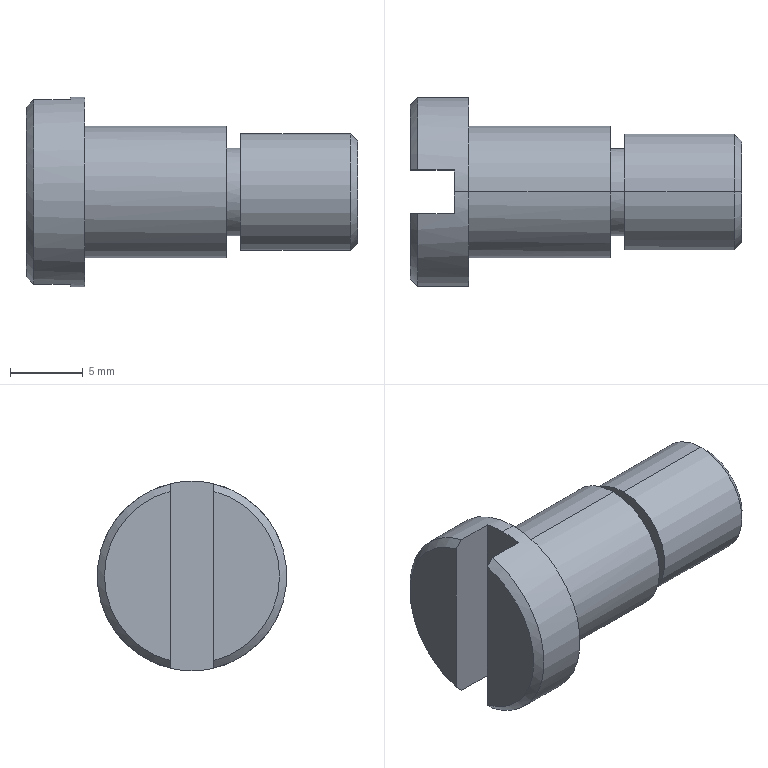Part | STEP file | 101000007761 | 1 solid | 21 faces | box 22.7 x 13 x 13 mm | volume 1455 mm3 | plane 9 | cylinder 8 | cone 4 | commonest cylinder face diameters 6 x2 8 x2 9 x2 13 x2
STEP:
#1=CARTESIAN_POINT('',(-23.823,0.,-3.5));
#2=VERTEX_POINT('',#1);
#3=CARTESIAN_POINT('',(-23.823,0.,3.5));
#4=VERTEX_POINT('',#3);
#5=CARTESIAN_POINT('',(-23.823,0.,0.));
#6=DIRECTION('',(-1.,0.,0.));
#7=AXIS2_PLACEMENT_3D('',#5,#6,$);
#8=CIRCLE('',#7,3.5);
#9=EDGE_CURVE('',#2,#4,#8,.F.);
#10=ORIENTED_EDGE('',*,*,#9,.F.);
#11=CARTESIAN_POINT('',(-24.323,0.,-4.));
#12=VERTEX_POINT('',#11);
#13=CARTESIAN_POINT('',(-353575.714,0.,-353555.391));
#14=DIRECTION('',(-0.7071,0.,-0.7071));
#15=VECTOR('',#14,1.);
#16=LINE('',#13,#15);
#17=EDGE_CURVE('',#2,#12,#16,.T.);
#18=ORIENTED_EDGE('',*,*,#17,.T.);
#19=CARTESIAN_POINT('',(-24.323,0.,4.));
#20=VERTEX_POINT('',#19);
#21=CARTESIAN_POINT('',(-24.323,0.,0.));
#22=DIRECTION('',(-1.,0.,0.));
#23=AXIS2_PLACEMENT_3D('',#21,#22,$);
#24=CIRCLE('',#23,4.);
#25=EDGE_CURVE('',#20,#12,#24,.T.);
#26=ORIENTED_EDGE('',*,*,#25,.F.);
#27=CARTESIAN_POINT('',(-353575.714,0.,353555.391));
#28=DIRECTION('',(-0.7071,0.,0.7071));
#29=VECTOR('',#28,1.);
#30=LINE('',#27,#29);
#31=EDGE_CURVE('',#4,#20,#30,.T.);
#32=ORIENTED_EDGE('',*,*,#31,.F.);
#33=EDGE_LOOP('',(#10,#18,#26,#32));
#34=FACE_OUTER_BOUND('',#33,.T.);
#35=CARTESIAN_POINT('',(-24.323,0.,0.));
#36=DIRECTION('',(-1.,0.,0.));
#37=DIRECTION('',(0.,0.,1.));
#38=AXIS2_PLACEMENT_3D('',#35,#36,#37);
#39=CONICAL_SURFACE('',#38,4.,0.7854);
#40=ADVANCED_FACE('',(#34),#39,.T.);
#41=CARTESIAN_POINT('',(-23.823,0.,3.5));
#42=CARTESIAN_POINT('',(-23.823,-0.3666,3.5));
#43=CARTESIAN_POINT('',(-23.823,-0.7332,3.452));
#44=CARTESIAN_POINT('',(-23.823,-1.091,3.356));
#45=CARTESIAN_POINT('',(-23.823,-1.774,3.072));
#46=CARTESIAN_POINT('',(-23.823,-2.361,2.623));
#47=CARTESIAN_POINT('',(-23.823,-2.624,2.36));
#48=CARTESIAN_POINT('',(-23.823,-3.073,1.773));
#49=CARTESIAN_POINT('',(-23.823,-3.356,1.09));
#50=CARTESIAN_POINT('',(-23.823,-3.452,0.7319));
#51=CARTESIAN_POINT('',(-23.823,-3.548,-0.001322));
#52=CARTESIAN_POINT('',(-23.823,-3.452,-0.7345));
#53=CARTESIAN_POINT('',(-23.823,-3.356,-1.093));
#54=CARTESIAN_POINT('',(-23.823,-3.072,-1.776));
#55=CARTESIAN_POINT('',(-23.823,-2.622,-2.362));
#56=CARTESIAN_POINT('',(-23.823,-2.359,-2.624));
#57=CARTESIAN_POINT('',(-23.823,-1.773,-3.073));
#58=CARTESIAN_POINT('',(-23.823,-1.09,-3.356));
#59=CARTESIAN_POINT('',(-23.823,-0.7322,-3.452));
#60=CARTESIAN_POINT('',(-23.823,-0.3661,-3.5));
#61=CARTESIAN_POINT('',(-23.823,0.,-3.5));
#62=B_SPLINE_CURVE_WITH_KNOTS('',5,(#41,#42,#43,#44,#45,#46,#47,#48,#49,#50,#51,#52,#53,#54,#55,#56,#57,#58,#59,#60,#61),.UNSPECIFIED.,.F.,.U.,(6,3,3,3,3,3,6),(0.,2.592,5.185,7.777,10.369,12.961,15.55),.UNSPECIFIED.);
#63=EDGE_CURVE('',#4,#2,#62,.T.);
#64=ORIENTED_EDGE('',*,*,#63,.T.);
#65=ORIENTED_EDGE('',*,*,#9,.T.);
#66=EDGE_LOOP('',(#64,#65));
#67=FACE_OUTER_BOUND('',#66,.T.);
#68=CARTESIAN_POINT('',(-23.823,4.,0.));
#69=DIRECTION('',(-1.,0.,0.));
#70=DIRECTION('',(0.,0.,1.));
#71=AXIS2_PLACEMENT_3D('',#68,#69,#70);
#72=PLANE('',#71);
#73=ADVANCED_FACE('',(#67),#72,.F.);
#74=ORIENTED_EDGE('',*,*,#17,.F.);
#75=ORIENTED_EDGE('',*,*,#63,.F.);
#76=ORIENTED_EDGE('',*,*,#31,.T.);
#77=CARTESIAN_POINT('',(-24.323,0.,0.));
#78=DIRECTION('',(-1.,0.,0.));
#79=AXIS2_PLACEMENT_3D('',#77,#78,$);
#80=CIRCLE('',#79,4.);
#81=EDGE_CURVE('',#12,#20,#80,.T.);
#82=ORIENTED_EDGE('',*,*,#81,.F.);
#83=EDGE_LOOP('',(#74,#75,#76,#82));
#84=FACE_OUTER_BOUND('',#83,.T.);
#85=CARTESIAN_POINT('',(-24.323,0.,0.));
#86=DIRECTION('',(-1.,0.,0.));
#87=DIRECTION('',(0.,0.,-1.));
#88=AXIS2_PLACEMENT_3D('',#85,#86,#87);
#89=CONICAL_SURFACE('',#88,4.,0.7854);
#90=ADVANCED_FACE('',(#84),#89,.T.);
#91=ORIENTED_EDGE('',*,*,#25,.T.);
#92=CARTESIAN_POINT('',(-31.823,0.,-4.));
#93=VERTEX_POINT('',#92);
#94=CARTESIAN_POINT('',(-55.053,0.,-4.));
#95=DIRECTION('',(-1.,0.,0.));
#96=VECTOR('',#95,1.);
#97=LINE('',#94,#96);
#98=EDGE_CURVE('',#12,#93,#97,.T.);
#99=ORIENTED_EDGE('',*,*,#98,.T.);
#100=CARTESIAN_POINT('',(-31.823,0.,4.));
#101=VERTEX_POINT('',#100);
#102=CARTESIAN_POINT('',(-31.823,0.,0.));
#103=DIRECTION('',(-1.,0.,0.));
#104=AXIS2_PLACEMENT_3D('',#102,#103,$);
#105=CIRCLE('',#104,4.);
#106=EDGE_CURVE('',#101,#93,#105,.T.);
#107=ORIENTED_EDGE('',*,*,#106,.F.);
#108=CARTESIAN_POINT('',(-55.053,0.,4.));
#109=DIRECTION('',(-1.,0.,0.));
#110=VECTOR('',#109,1.);
#111=LINE('',#108,#110);
#112=EDGE_CURVE('',#20,#101,#111,.T.);
#113=ORIENTED_EDGE('',*,*,#112,.F.);
#114=EDGE_LOOP('',(#91,#99,#107,#113));
#115=FACE_OUTER_BOUND('',#114,.T.);
#116=CARTESIAN_POINT('',(-55.053,0.,0.));
#117=DIRECTION('',(-1.,0.,0.));
#118=DIRECTION('',(0.,0.,1.));
#119=AXIS2_PLACEMENT_3D('',#116,#117,#118);
#120=CYLINDRICAL_SURFACE('',#119,4.);
#121=ADVANCED_FACE('',(#115),#120,.T.);
#122=ORIENTED_EDGE('',*,*,#98,.F.);
#123=ORIENTED_EDGE('',*,*,#81,.T.);
#124=ORIENTED_EDGE('',*,*,#112,.T.);
#125=CARTESIAN_POINT('',(-31.823,0.,-4.));
#126=CARTESIAN_POINT('',(-31.823,-0.6283,-4.));
#127=CARTESIAN_POINT('',(-31.823,-1.257,-3.877));
#128=CARTESIAN_POINT('',(-31.823,-1.853,-3.63));
#129=CARTESIAN_POINT('',(-31.823,-2.916,-2.916));
#130=CARTESIAN_POINT('',(-31.823,-3.63,-1.853));
#131=CARTESIAN_POINT('',(-31.823,-3.877,-1.257));
#132=CARTESIAN_POINT('',(-31.823,-4.123,0.));
#133=CARTESIAN_POINT('',(-31.823,-3.877,1.257));
#134=CARTESIAN_POINT('',(-31.823,-3.63,1.853));
#135=CARTESIAN_POINT('',(-31.823,-2.916,2.916));
#136=CARTESIAN_POINT('',(-31.823,-1.853,3.63));
#137=CARTESIAN_POINT('',(-31.823,-1.257,3.877));
#138=CARTESIAN_POINT('',(-31.823,-0.6283,4.));
#139=CARTESIAN_POINT('',(-31.823,0.,4.));
#140=B_SPLINE_CURVE_WITH_KNOTS('',5,(#125,#126,#127,#128,#129,#130,#131,#132,#133,#134,#135,#136,#137,#138,#139),.UNSPECIFIED.,.F.,.U.,(6,3,3,3,6),(-6.283,-3.142,0.,3.142,6.283),.UNSPECIFIED.);
#141=EDGE_CURVE('',#93,#101,#140,.T.);
#142=ORIENTED_EDGE('',*,*,#141,.F.);
#143=EDGE_LOOP('',(#122,#123,#124,#142));
#144=FACE_OUTER_BOUND('',#143,.T.);
#145=CARTESIAN_POINT('',(-55.053,0.,0.));
#146=DIRECTION('',(-1.,0.,0.));
#147=DIRECTION('',(0.,0.,-1.));
#148=AXIS2_PLACEMENT_3D('',#145,#146,#147);
#149=CYLINDRICAL_SURFACE('',#148,4.);
#150=ADVANCED_FACE('',(#144),#149,.T.);
#151=ORIENTED_EDGE('',*,*,#106,.T.);
#152=ORIENTED_EDGE('',*,*,#141,.T.);
#153=EDGE_LOOP('',(#151,#152));
#154=FACE_OUTER_BOUND('',#153,.T.);
#155=CARTESIAN_POINT('',(-31.823,0.,3.));
#156=VERTEX_POINT('',#155);
#157=CARTESIAN_POINT('',(-31.823,0.,-3.));
#158=VERTEX_POINT('',#157);
#159=CARTESIAN_POINT('',(-31.823,0.,3.));
#160=CARTESIAN_POINT('',(-31.823,0.3394,3.));
#161=CARTESIAN_POINT('',(-31.823,0.6788,2.952));
#162=CARTESIAN_POINT('',(-31.823,1.009,2.856));
#163=CARTESIAN_POINT('',(-31.823,1.634,2.573));
#164=CARTESIAN_POINT('',(-31.823,2.155,2.128));
#165=CARTESIAN_POINT('',(-31.823,2.383,1.87));
#166=CARTESIAN_POINT('',(-31.823,2.758,1.297));
#167=CARTESIAN_POINT('',(-31.823,2.96,0.6415));
#168=CARTESIAN_POINT('',(-31.823,3.014,0.3017));
#169=CARTESIAN_POINT('',(-31.823,3.024,-0.3838));
#170=CARTESIAN_POINT('',(-31.823,2.843,-1.045));
#171=CARTESIAN_POINT('',(-31.823,2.706,-1.361));
#172=CARTESIAN_POINT('',(-31.823,2.347,-1.945));
#173=CARTESIAN_POINT('',(-31.823,1.84,-2.406));
#174=CARTESIAN_POINT('',(-31.823,1.555,-2.599));
#175=CARTESIAN_POINT('',(-31.823,1.077,-2.833));
#176=CARTESIAN_POINT('',(-31.823,0.5622,-2.956));
#177=CARTESIAN_POINT('',(-31.823,0.3758,-2.985));
#178=CARTESIAN_POINT('',(-31.823,0.1879,-3.));
#179=CARTESIAN_POINT('',(-31.823,0.,-3.));
#180=B_SPLINE_CURVE_WITH_KNOTS('',5,(#159,#160,#161,#162,#163,#164,#165,#166,#167,#168,#169,#170,#171,#172,#173,#174,#175,#176,#177,#178,#179),.UNSPECIFIED.,.F.,.U.,(6,3,3,3,3,3,6),(0.,2.4,4.8,7.2,9.6,12.,13.328),.UNSPECIFIED.);
#181=EDGE_CURVE('',#156,#158,#180,.T.);
#182=ORIENTED_EDGE('',*,*,#181,.F.);
#183=CARTESIAN_POINT('',(-31.823,0.,-3.));
#184=CARTESIAN_POINT('',(-31.823,-0.3394,-3.));
#185=CARTESIAN_POINT('',(-31.823,-0.6788,-2.952));
#186=CARTESIAN_POINT('',(-31.823,-1.009,-2.856));
#187=CARTESIAN_POINT('',(-31.823,-1.634,-2.573));
#188=CARTESIAN_POINT('',(-31.823,-2.155,-2.128));
#189=CARTESIAN_POINT('',(-31.823,-2.383,-1.87));
#190=CARTESIAN_POINT('',(-31.823,-2.758,-1.297));
#191=CARTESIAN_POINT('',(-31.823,-2.96,-0.6415));
#192=CARTESIAN_POINT('',(-31.823,-3.014,-0.3017));
#193=CARTESIAN_POINT('',(-31.823,-3.024,0.3838));
#194=CARTESIAN_POINT('',(-31.823,-2.843,1.045));
#195=CARTESIAN_POINT('',(-31.823,-2.706,1.361));
#196=CARTESIAN_POINT('',(-31.823,-2.347,1.945));
#197=CARTESIAN_POINT('',(-31.823,-1.84,2.406));
#198=CARTESIAN_POINT('',(-31.823,-1.555,2.599));
#199=CARTESIAN_POINT('',(-31.823,-1.077,2.833));
#200=CARTESIAN_POINT('',(-31.823,-0.5622,2.956));
#201=CARTESIAN_POINT('',(-31.823,-0.3758,2.985));
#202=CARTESIAN_POINT('',(-31.823,-0.1879,3.));
#203=CARTESIAN_POINT('',(-31.823,0.,3.));
#204=B_SPLINE_CURVE_WITH_KNOTS('',5,(#183,#184,#185,#186,#187,#188,#189,#190,#191,#192,#193,#194,#195,#196,#197,#198,#199,#200,#201,#202,#203),.UNSPECIFIED.,.F.,.U.,(6,3,3,3,3,3,6),(0.,2.4,4.8,7.2,9.6,12.,13.328),.UNSPECIFIED.);
#205=EDGE_CURVE('',#158,#156,#204,.T.);
#206=ORIENTED_EDGE('',*,*,#205,.F.);
#207=EDGE_LOOP('',(#182,#206));
#208=FACE_BOUND('',#207,.T.);
#209=CARTESIAN_POINT('',(-31.823,3.,0.));
#210=DIRECTION('',(1.,0.,0.));
#211=DIRECTION('',(0.,0.,-1.));
#212=AXIS2_PLACEMENT_3D('',#209,#210,#211);
#213=PLANE('',#212);
#214=ADVANCED_FACE('',(#154,#208),#213,.F.);
#215=ORIENTED_EDGE('',*,*,#181,.T.);
#216=CARTESIAN_POINT('',(-32.823,0.,-3.));
#217=VERTEX_POINT('',#216);
#218=CARTESIAN_POINT('',(-55.053,0.,-3.));
#219=DIRECTION('',(-1.,0.,0.));
#220=VECTOR('',#219,1.);
#221=LINE('',#218,#220);
#222=EDGE_CURVE('',#158,#217,#221,.T.);
#223=ORIENTED_EDGE('',*,*,#222,.T.);
#224=CARTESIAN_POINT('',(-32.823,0.,3.));
#225=VERTEX_POINT('',#224);
#226=CARTESIAN_POINT('',(-32.823,0.,0.));
#227=DIRECTION('',(-1.,0.,0.));
#228=AXIS2_PLACEMENT_3D('',#226,#227,$);
#229=CIRCLE('',#228,3.);
#230=EDGE_CURVE('',#225,#217,#229,.T.);
#231=ORIENTED_EDGE('',*,*,#230,.F.);
#232=CARTESIAN_POINT('',(-55.053,0.,3.));
#233=DIRECTION('',(-1.,0.,0.));
#234=VECTOR('',#233,1.);
#235=LINE('',#232,#234);
#236=EDGE_CURVE('',#156,#225,#235,.T.);
#237=ORIENTED_EDGE('',*,*,#236,.F.);
#238=EDGE_LOOP('',(#215,#223,#231,#237));
#239=FACE_OUTER_BOUND('',#238,.T.);
#240=CARTESIAN_POINT('',(-55.053,0.,0.));
#241=DIRECTION('',(-1.,0.,0.));
#242=DIRECTION('',(0.,0.,1.));
#243=AXIS2_PLACEMENT_3D('',#240,#241,#242);
#244=CYLINDRICAL_SURFACE('',#243,3.);
#245=ADVANCED_FACE('',(#239),#244,.T.);
#246=ORIENTED_EDGE('',*,*,#222,.F.);
#247=ORIENTED_EDGE('',*,*,#205,.T.);
#248=ORIENTED_EDGE('',*,*,#236,.T.);
#249=CARTESIAN_POINT('',(-32.823,0.,-3.));
#250=CARTESIAN_POINT('',(-32.823,-0.9425,-3.));
#251=CARTESIAN_POINT('',(-32.823,-1.885,-2.63));
#252=CARTESIAN_POINT('',(-32.823,-2.63,-1.885));
#253=CARTESIAN_POINT('',(-32.823,-3.37,0.));
#254=CARTESIAN_POINT('',(-32.823,-2.63,1.885));
#255=CARTESIAN_POINT('',(-32.823,-1.885,2.63));
#256=CARTESIAN_POINT('',(-32.823,-0.9425,3.));
#257=CARTESIAN_POINT('',(-32.823,0.,3.));
#258=B_SPLINE_CURVE_WITH_KNOTS('',5,(#249,#250,#251,#252,#253,#254,#255,#256,#257),.UNSPECIFIED.,.F.,.U.,(6,3,6),(-4.712,0.,4.712),.UNSPECIFIED.);
#259=EDGE_CURVE('',#217,#225,#258,.T.);
#260=ORIENTED_EDGE('',*,*,#259,.F.);
#261=EDGE_LOOP('',(#246,#247,#248,#260));
#262=FACE_OUTER_BOUND('',#261,.T.);
#263=CARTESIAN_POINT('',(-55.053,0.,0.));
#264=DIRECTION('',(-1.,0.,0.));
#265=DIRECTION('',(0.,0.,-1.));
#266=AXIS2_PLACEMENT_3D('',#263,#264,#265);
#267=CYLINDRICAL_SURFACE('',#266,3.);
#268=ADVANCED_FACE('',(#262),#267,.T.);
#269=CARTESIAN_POINT('',(-32.823,0.,4.5));
#270=VERTEX_POINT('',#269);
#271=CARTESIAN_POINT('',(-32.823,0.,-4.5));
#272=VERTEX_POINT('',#271);
#273=CARTESIAN_POINT('',(-32.823,0.,0.));
#274=DIRECTION('',(-1.,0.,0.));
#275=AXIS2_PLACEMENT_3D('',#273,#274,$);
#276=CIRCLE('',#275,4.5);
#277=EDGE_CURVE('',#270,#272,#276,.T.);
#278=ORIENTED_EDGE('',*,*,#277,.F.);
#279=CARTESIAN_POINT('',(-32.823,0.,0.));
#280=DIRECTION('',(-1.,0.,0.));
#281=AXIS2_PLACEMENT_3D('',#279,#280,$);
#282=CIRCLE('',#281,4.5);
#283=EDGE_CURVE('',#272,#270,#282,.T.);
#284=ORIENTED_EDGE('',*,*,#283,.F.);
#285=EDGE_LOOP('',(#278,#284));
#286=FACE_OUTER_BOUND('',#285,.T.);
#287=ORIENTED_EDGE('',*,*,#230,.T.);
#288=ORIENTED_EDGE('',*,*,#259,.T.);
#289=EDGE_LOOP('',(#287,#288));
#290=FACE_BOUND('',#289,.T.);
#291=CARTESIAN_POINT('',(-32.823,4.5,0.));
#292=DIRECTION('',(-1.,0.,0.));
#293=DIRECTION('',(0.,0.,1.));
#294=AXIS2_PLACEMENT_3D('',#291,#292,#293);
#295=PLANE('',#294);
#296=ADVANCED_FACE('',(#286,#290),#295,.F.);
#297=ORIENTED_EDGE('',*,*,#277,.T.);
#298=CARTESIAN_POINT('',(-42.523,0.,-4.5));
#299=VERTEX_POINT('',#298);
#300=CARTESIAN_POINT('',(-55.053,0.,-4.5));
#301=DIRECTION('',(-1.,0.,0.));
#302=VECTOR('',#301,1.);
#303=LINE('',#300,#302);
#304=EDGE_CURVE('',#272,#299,#303,.T.);
#305=ORIENTED_EDGE('',*,*,#304,.T.);
#306=CARTESIAN_POINT('',(-42.523,0.,4.5));
#307=VERTEX_POINT('',#306);
#308=CARTESIAN_POINT('',(-42.523,0.,0.));
#309=DIRECTION('',(-1.,0.,0.));
#310=AXIS2_PLACEMENT_3D('',#308,#309,$);
#311=CIRCLE('',#310,4.5);
#312=EDGE_CURVE('',#307,#299,#311,.T.);
#313=ORIENTED_EDGE('',*,*,#312,.F.);
#314=CARTESIAN_POINT('',(-55.053,0.,4.5));
#315=DIRECTION('',(-1.,0.,0.));
#316=VECTOR('',#315,1.);
#317=LINE('',#314,#316);
#318=EDGE_CURVE('',#270,#307,#317,.T.);
#319=ORIENTED_EDGE('',*,*,#318,.F.);
#320=EDGE_LOOP('',(#297,#305,#313,#319));
#321=FACE_OUTER_BOUND('',#320,.T.);
#322=CARTESIAN_POINT('',(-55.053,0.,0.));
#323=DIRECTION('',(-1.,0.,0.));
#324=DIRECTION('',(0.,0.,1.));
#325=AXIS2_PLACEMENT_3D('',#322,#323,#324);
#326=CYLINDRICAL_SURFACE('',#325,4.5);
#327=ADVANCED_FACE('',(#321),#326,.T.);
#328=ORIENTED_EDGE('',*,*,#304,.F.);
#329=ORIENTED_EDGE('',*,*,#283,.T.);
#330=ORIENTED_EDGE('',*,*,#318,.T.);
#331=CARTESIAN_POINT('',(-42.523,0.,-4.5));
#332=CARTESIAN_POINT('',(-42.523,-0.7069,-4.5));
#333=CARTESIAN_POINT('',(-42.523,-1.414,-4.361));
#334=CARTESIAN_POINT('',(-42.523,-2.084,-4.083));
#335=CARTESIAN_POINT('',(-42.523,-3.28,-3.28));
#336=CARTESIAN_POINT('',(-42.523,-4.083,-2.084));
#337=CARTESIAN_POINT('',(-42.523,-4.361,-1.414));
#338=CARTESIAN_POINT('',(-42.523,-4.639,0.));
#339=CARTESIAN_POINT('',(-42.523,-4.361,1.414));
#340=CARTESIAN_POINT('',(-42.523,-4.083,2.084));
#341=CARTESIAN_POINT('',(-42.523,-3.28,3.28));
#342=CARTESIAN_POINT('',(-42.523,-2.084,4.083));
#343=CARTESIAN_POINT('',(-42.523,-1.414,4.361));
#344=CARTESIAN_POINT('',(-42.523,-0.7069,4.5));
#345=CARTESIAN_POINT('',(-42.523,0.,4.5));
#346=B_SPLINE_CURVE_WITH_KNOTS('',5,(#331,#332,#333,#334,#335,#336,#337,#338,#339,#340,#341,#342,#343,#344,#345),.UNSPECIFIED.,.F.,.U.,(6,3,3,3,6),(-7.069,-3.534,0.,3.534,7.069),.UNSPECIFIED.);
#347=EDGE_CURVE('',#299,#307,#346,.T.);
#348=ORIENTED_EDGE('',*,*,#347,.F.);
#349=EDGE_LOOP('',(#328,#329,#330,#348));
#350=FACE_OUTER_BOUND('',#349,.T.);
#351=CARTESIAN_POINT('',(-55.053,0.,0.));
#352=DIRECTION('',(-1.,0.,0.));
#353=DIRECTION('',(0.,0.,-1.));
#354=AXIS2_PLACEMENT_3D('',#351,#352,#353);
#355=CYLINDRICAL_SURFACE('',#354,4.5);
#356=ADVANCED_FACE('',(#350),#355,.T.);
#357=CARTESIAN_POINT('',(-42.523,0.,6.5));
#358=VERTEX_POINT('',#357);
#359=CARTESIAN_POINT('',(-42.523,0.,-6.5));
#360=VERTEX_POINT('',#359);
#361=CARTESIAN_POINT('',(-42.523,0.,0.));
#362=DIRECTION('',(-1.,0.,0.));
#363=AXIS2_PLACEMENT_3D('',#361,#362,$);
#364=CIRCLE('',#363,6.5);
#365=EDGE_CURVE('',#358,#360,#364,.T.);
#366=ORIENTED_EDGE('',*,*,#365,.F.);
#367=CARTESIAN_POINT('',(-42.523,0.,0.));
#368=DIRECTION('',(-1.,0.,0.));
#369=AXIS2_PLACEMENT_3D('',#367,#368,$);
#370=CIRCLE('',#369,6.5);
#371=EDGE_CURVE('',#360,#358,#370,.T.);
#372=ORIENTED_EDGE('',*,*,#371,.F.);
#373=EDGE_LOOP('',(#366,#372));
#374=FACE_OUTER_BOUND('',#373,.T.);
#375=ORIENTED_EDGE('',*,*,#312,.T.);
#376=ORIENTED_EDGE('',*,*,#347,.T.);
#377=EDGE_LOOP('',(#375,#376));
#378=FACE_BOUND('',#377,.T.);
#379=CARTESIAN_POINT('',(-42.523,6.5,0.));
#380=DIRECTION('',(-1.,0.,0.));
#381=DIRECTION('',(0.,0.,1.));
#382=AXIS2_PLACEMENT_3D('',#379,#380,#381);
#383=PLANE('',#382);
#384=ADVANCED_FACE('',(#374,#378),#383,.F.);
#385=ORIENTED_EDGE('',*,*,#365,.T.);
#386=CARTESIAN_POINT('',(-43.523,0.,-6.5));
#387=VERTEX_POINT('',#386);
#388=CARTESIAN_POINT('',(-55.053,0.,-6.5));
#389=DIRECTION('',(-1.,0.,0.));
#390=VECTOR('',#389,1.);
#391=LINE('',#388,#390);
#392=EDGE_CURVE('',#360,#387,#391,.T.);
#393=ORIENTED_EDGE('',*,*,#392,.T.);
#394=CARTESIAN_POINT('',(-43.523,1.5,-6.325));
#395=VERTEX_POINT('',#394);
#396=CARTESIAN_POINT('',(-43.523,0.,0.));
#397=DIRECTION('',(-1.,0.,0.));
#398=AXIS2_PLACEMENT_3D('',#396,#397,$);
#399=CIRCLE('',#398,6.5);
#400=EDGE_CURVE('',#387,#395,#399,.F.);
#401=ORIENTED_EDGE('',*,*,#400,.T.);
#402=CARTESIAN_POINT('',(-46.023,1.5,-6.325));
#403=VERTEX_POINT('',#402);
#404=CARTESIAN_POINT('',(-55.053,1.5,-6.325));
#405=DIRECTION('',(-1.,0.,0.));
#406=VECTOR('',#405,1.);
#407=LINE('',#404,#406);
#408=EDGE_CURVE('',#395,#403,#407,.T.);
#409=ORIENTED_EDGE('',*,*,#408,.T.);
#410=CARTESIAN_POINT('',(-46.023,1.5,6.325));
#411=VERTEX_POINT('',#410);
#412=CARTESIAN_POINT('',(-46.023,0.,0.));
#413=DIRECTION('',(-1.,0.,0.));
#414=AXIS2_PLACEMENT_3D('',#412,#413,$);
#415=CIRCLE('',#414,6.5);
#416=EDGE_CURVE('',#403,#411,#415,.F.);
#417=ORIENTED_EDGE('',*,*,#416,.T.);
#418=CARTESIAN_POINT('',(-43.523,1.5,6.325));
#419=VERTEX_POINT('',#418);
#420=CARTESIAN_POINT('',(-55.053,1.5,6.325));
#421=DIRECTION('',(-1.,0.,0.));
#422=VECTOR('',#421,1.);
#423=LINE('',#420,#422);
#424=EDGE_CURVE('',#411,#419,#423,.F.);
#425=ORIENTED_EDGE('',*,*,#424,.T.);
#426=CARTESIAN_POINT('',(-43.523,0.,6.5));
#427=VERTEX_POINT('',#426);
#428=CARTESIAN_POINT('',(-43.523,0.,0.));
#429=DIRECTION('',(-1.,0.,0.));
#430=AXIS2_PLACEMENT_3D('',#428,#429,$);
#431=CIRCLE('',#430,6.5);
#432=EDGE_CURVE('',#419,#427,#431,.F.);
#433=ORIENTED_EDGE('',*,*,#432,.T.);
#434=CARTESIAN_POINT('',(-55.053,0.,6.5));
#435=DIRECTION('',(-1.,0.,0.));
#436=VECTOR('',#435,1.);
#437=LINE('',#434,#436);
#438=EDGE_CURVE('',#358,#427,#437,.T.);
#439=ORIENTED_EDGE('',*,*,#438,.F.);
#440=EDGE_LOOP('',(#385,#393,#401,#409,#417,#425,#433,#439));
#441=FACE_OUTER_BOUND('',#440,.T.);
#442=CARTESIAN_POINT('',(-55.053,0.,0.));
#443=DIRECTION('',(-1.,0.,0.));
#444=DIRECTION('',(0.,0.,1.));
#445=AXIS2_PLACEMENT_3D('',#442,#443,#444);
#446=CYLINDRICAL_SURFACE('',#445,6.5);
#447=ADVANCED_FACE('',(#441),#446,.T.);
#448=ORIENTED_EDGE('',*,*,#392,.F.);
#449=ORIENTED_EDGE('',*,*,#371,.T.);
#450=ORIENTED_EDGE('',*,*,#438,.T.);
#451=CARTESIAN_POINT('',(-43.523,-1.5,6.325));
#452=VERTEX_POINT('',#451);
#453=CARTESIAN_POINT('',(-43.523,0.,0.));
#454=DIRECTION('',(-1.,0.,0.));
#455=AXIS2_PLACEMENT_3D('',#453,#454,$);
#456=CIRCLE('',#455,6.5);
#457=EDGE_CURVE('',#427,#452,#456,.F.);
#458=ORIENTED_EDGE('',*,*,#457,.T.);
#459=CARTESIAN_POINT('',(-46.023,-1.5,6.325));
#460=VERTEX_POINT('',#459);
#461=CARTESIAN_POINT('',(-55.053,-1.5,6.325));
#462=DIRECTION('',(-1.,0.,0.));
#463=VECTOR('',#462,1.);
#464=LINE('',#461,#463);
#465=EDGE_CURVE('',#452,#460,#464,.T.);
#466=ORIENTED_EDGE('',*,*,#465,.T.);
#467=CARTESIAN_POINT('',(-46.023,-1.5,-6.325));
#468=VERTEX_POINT('',#467);
#469=CARTESIAN_POINT('',(-46.023,0.,0.));
#470=DIRECTION('',(-1.,0.,0.));
#471=AXIS2_PLACEMENT_3D('',#469,#470,$);
#472=CIRCLE('',#471,6.5);
#473=EDGE_CURVE('',#460,#468,#472,.F.);
#474=ORIENTED_EDGE('',*,*,#473,.T.);
#475=CARTESIAN_POINT('',(-43.523,-1.5,-6.325));
#476=VERTEX_POINT('',#475);
#477=CARTESIAN_POINT('',(-55.053,-1.5,-6.325));
#478=DIRECTION('',(-1.,0.,0.));
#479=VECTOR('',#478,1.);
#480=LINE('',#477,#479);
#481=EDGE_CURVE('',#468,#476,#480,.F.);
#482=ORIENTED_EDGE('',*,*,#481,.T.);
#483=CARTESIAN_POINT('',(-43.523,-1.5,-6.325));
#484=CARTESIAN_POINT('',(-43.523,-1.009,-6.441));
#485=CARTESIAN_POINT('',(-43.523,-0.5045,-6.5));
#486=CARTESIAN_POINT('',(-43.523,0.,-6.5));
#487=B_SPLINE_CURVE_WITH_KNOTS('',3,(#483,#484,#485,#486),.UNSPECIFIED.,.F.,.U.,(4,4),(-0.7568,0.7568),.UNSPECIFIED.);
#488=EDGE_CURVE('',#476,#387,#487,.T.);
#489=ORIENTED_EDGE('',*,*,#488,.T.);
#490=EDGE_LOOP('',(#448,#449,#450,#458,#466,#474,#482,#489));
#491=FACE_OUTER_BOUND('',#490,.T.);
#492=CARTESIAN_POINT('',(-55.053,0.,0.));
#493=DIRECTION('',(-1.,0.,0.));
#494=DIRECTION('',(0.,0.,-1.));
#495=AXIS2_PLACEMENT_3D('',#492,#493,#494);
#496=CYLINDRICAL_SURFACE('',#495,6.5);
#497=ADVANCED_FACE('',(#491),#496,.T.);
#498=CARTESIAN_POINT('',(-43.523,1.5,0.));
#499=DIRECTION('',(0.,0.,1.));
#500=VECTOR('',#499,1.);
#501=LINE('',#498,#500);
#502=EDGE_CURVE('',#395,#419,#501,.T.);
#503=ORIENTED_EDGE('',*,*,#502,.F.);
#504=ORIENTED_EDGE('',*,*,#400,.F.);
#505=ORIENTED_EDGE('',*,*,#488,.F.);
#506=CARTESIAN_POINT('',(-43.523,-1.5,0.));
#507=DIRECTION('',(0.,0.,1.));
#508=VECTOR('',#507,1.);
#509=LINE('',#506,#508);
#510=EDGE_CURVE('',#476,#452,#509,.T.);
#511=ORIENTED_EDGE('',*,*,#510,.T.);
#512=ORIENTED_EDGE('',*,*,#457,.F.);
#513=ORIENTED_EDGE('',*,*,#432,.F.);
#514=EDGE_LOOP('',(#503,#504,#505,#511,#512,#513));
#515=FACE_OUTER_BOUND('',#514,.T.);
#516=CARTESIAN_POINT('',(-43.523,1.5,-6.5));
#517=DIRECTION('',(1.,0.,0.));
#518=DIRECTION('',(0.,0.,-1.));
#519=AXIS2_PLACEMENT_3D('',#516,#517,#518);
#520=PLANE('',#519);
#521=ADVANCED_FACE('',(#515),#520,.F.);
#522=CARTESIAN_POINT('',(-46.523,1.5,-5.809));
#523=VERTEX_POINT('',#522);
#524=CARTESIAN_POINT('',(-46.523,1.5,5.809));
#525=VERTEX_POINT('',#524);
#526=CARTESIAN_POINT('',(-46.523,1.5,0.));
#527=DIRECTION('',(0.,0.,1.));
#528=VECTOR('',#527,1.);
#529=LINE('',#526,#528);
#530=EDGE_CURVE('',#523,#525,#529,.T.);
#531=ORIENTED_EDGE('',*,*,#530,.F.);
#532=CARTESIAN_POINT('',(-46.523,1.5,-5.809));
#533=CARTESIAN_POINT('',(-46.424,1.5,-5.913));
#534=CARTESIAN_POINT('',(-46.324,1.5,-6.016));
#535=CARTESIAN_POINT('',(-46.224,1.5,-6.119));
#536=CARTESIAN_POINT('',(-46.124,1.5,-6.222));
#537=CARTESIAN_POINT('',(-46.023,1.5,-6.325));
#538=B_SPLINE_CURVE_WITH_KNOTS('',5,(#532,#533,#534,#535,#536,#537),.UNSPECIFIED.,.F.,.U.,(6,6),(0.,1.015),.UNSPECIFIED.);
#539=EDGE_CURVE('',#523,#403,#538,.T.);
#540=ORIENTED_EDGE('',*,*,#539,.T.);
#541=ORIENTED_EDGE('',*,*,#408,.F.);
#542=ORIENTED_EDGE('',*,*,#502,.T.);
#543=ORIENTED_EDGE('',*,*,#424,.F.);
#544=CARTESIAN_POINT('',(-46.023,1.5,6.325));
#545=CARTESIAN_POINT('',(-46.124,1.5,6.222));
#546=CARTESIAN_POINT('',(-46.224,1.5,6.119));
#547=CARTESIAN_POINT('',(-46.324,1.5,6.016));
#548=CARTESIAN_POINT('',(-46.424,1.5,5.913));
#549=CARTESIAN_POINT('',(-46.523,1.5,5.809));
#550=B_SPLINE_CURVE_WITH_KNOTS('',5,(#544,#545,#546,#547,#548,#549),.UNSPECIFIED.,.F.,.U.,(6,6),(0.,1.015),.UNSPECIFIED.);
#551=EDGE_CURVE('',#411,#525,#550,.T.);
#552=ORIENTED_EDGE('',*,*,#551,.T.);
#553=EDGE_LOOP('',(#531,#540,#541,#542,#543,#552));
#554=FACE_OUTER_BOUND('',#553,.T.);
#555=CARTESIAN_POINT('',(-46.523,1.5,-6.5));
#556=DIRECTION('',(0.,1.,0.));
#557=DIRECTION('',(0.,0.,1.));
#558=AXIS2_PLACEMENT_3D('',#555,#556,#557);
#559=PLANE('',#558);
#560=ADVANCED_FACE('',(#554),#559,.F.);
#561=ORIENTED_EDGE('',*,*,#551,.F.);
#562=ORIENTED_EDGE('',*,*,#416,.F.);
#563=ORIENTED_EDGE('',*,*,#539,.F.);
#564=CARTESIAN_POINT('',(-46.523,0.,0.));
#565=DIRECTION('',(1.,0.,0.));
#566=AXIS2_PLACEMENT_3D('',#564,#565,$);
#567=CIRCLE('',#566,6.);
#568=EDGE_CURVE('',#525,#523,#567,.F.);
#569=ORIENTED_EDGE('',*,*,#568,.F.);
#570=EDGE_LOOP('',(#561,#562,#563,#569));
#571=FACE_OUTER_BOUND('',#570,.T.);
#572=CARTESIAN_POINT('',(-46.523,0.,0.));
#573=DIRECTION('',(1.,0.,0.));
#574=DIRECTION('',(0.,0.,-1.));
#575=AXIS2_PLACEMENT_3D('',#572,#573,#574);
#576=CONICAL_SURFACE('',#575,6.,0.7854);
#577=ADVANCED_FACE('',(#571),#576,.T.);
#578=CARTESIAN_POINT('',(-46.523,-1.5,-5.809));
#579=VERTEX_POINT('',#578);
#580=CARTESIAN_POINT('',(-46.523,-1.5,5.809));
#581=VERTEX_POINT('',#580);
#582=CARTESIAN_POINT('',(-46.523,-1.5,0.));
#583=DIRECTION('',(0.,0.,1.));
#584=VECTOR('',#583,1.);
#585=LINE('',#582,#584);
#586=EDGE_CURVE('',#579,#581,#585,.T.);
#587=ORIENTED_EDGE('',*,*,#586,.T.);
#588=CARTESIAN_POINT('',(-46.523,-1.5,5.809));
#589=CARTESIAN_POINT('',(-46.424,-1.5,5.913));
#590=CARTESIAN_POINT('',(-46.324,-1.5,6.016));
#591=CARTESIAN_POINT('',(-46.224,-1.5,6.119));
#592=CARTESIAN_POINT('',(-46.124,-1.5,6.222));
#593=CARTESIAN_POINT('',(-46.023,-1.5,6.325));
#594=B_SPLINE_CURVE_WITH_KNOTS('',5,(#588,#589,#590,#591,#592,#593),.UNSPECIFIED.,.F.,.U.,(6,6),(0.,1.015),.UNSPECIFIED.);
#595=EDGE_CURVE('',#581,#460,#594,.T.);
#596=ORIENTED_EDGE('',*,*,#595,.T.);
#597=ORIENTED_EDGE('',*,*,#465,.F.);
#598=ORIENTED_EDGE('',*,*,#510,.F.);
#599=ORIENTED_EDGE('',*,*,#481,.F.);
#600=CARTESIAN_POINT('',(-46.023,-1.5,-6.325));
#601=CARTESIAN_POINT('',(-46.124,-1.5,-6.222));
#602=CARTESIAN_POINT('',(-46.224,-1.5,-6.119));
#603=CARTESIAN_POINT('',(-46.324,-1.5,-6.016));
#604=CARTESIAN_POINT('',(-46.424,-1.5,-5.913));
#605=CARTESIAN_POINT('',(-46.523,-1.5,-5.809));
#606=B_SPLINE_CURVE_WITH_KNOTS('',5,(#600,#601,#602,#603,#604,#605),.UNSPECIFIED.,.F.,.U.,(6,6),(0.,1.015),.UNSPECIFIED.);
#607=EDGE_CURVE('',#468,#579,#606,.T.);
#608=ORIENTED_EDGE('',*,*,#607,.T.);
#609=EDGE_LOOP('',(#587,#596,#597,#598,#599,#608));
#610=FACE_OUTER_BOUND('',#609,.T.);
#611=CARTESIAN_POINT('',(-46.523,-1.5,-6.5));
#612=DIRECTION('',(0.,-1.,0.));
#613=DIRECTION('',(0.,0.,-1.));
#614=AXIS2_PLACEMENT_3D('',#611,#612,#613);
#615=PLANE('',#614);
#616=ADVANCED_FACE('',(#610),#615,.F.);
#617=ORIENTED_EDGE('',*,*,#607,.F.);
#618=ORIENTED_EDGE('',*,*,#473,.F.);
#619=ORIENTED_EDGE('',*,*,#595,.F.);
#620=CARTESIAN_POINT('',(-46.523,0.,0.));
#621=DIRECTION('',(1.,0.,0.));
#622=AXIS2_PLACEMENT_3D('',#620,#621,$);
#623=CIRCLE('',#622,6.);
#624=EDGE_CURVE('',#579,#581,#623,.F.);
#625=ORIENTED_EDGE('',*,*,#624,.F.);
#626=EDGE_LOOP('',(#617,#618,#619,#625));
#627=FACE_OUTER_BOUND('',#626,.T.);
#628=CARTESIAN_POINT('',(-46.523,0.,0.));
#629=DIRECTION('',(1.,0.,0.));
#630=DIRECTION('',(0.,0.,1.));
#631=AXIS2_PLACEMENT_3D('',#628,#629,#630);
#632=CONICAL_SURFACE('',#631,6.,0.7854);
#633=ADVANCED_FACE('',(#627),#632,.T.);
#634=ORIENTED_EDGE('',*,*,#530,.T.);
#635=ORIENTED_EDGE('',*,*,#568,.T.);
#636=EDGE_LOOP('',(#634,#635));
#637=FACE_OUTER_BOUND('',#636,.T.);
#638=CARTESIAN_POINT('',(-46.523,0.,0.));
#639=DIRECTION('',(1.,0.,0.));
#640=DIRECTION('',(0.,0.,-1.));
#641=AXIS2_PLACEMENT_3D('',#638,#639,#640);
#642=PLANE('',#641);
#643=ADVANCED_FACE('',(#637),#642,.F.);
#644=ORIENTED_EDGE('',*,*,#586,.F.);
#645=ORIENTED_EDGE('',*,*,#624,.T.);
#646=EDGE_LOOP('',(#644,#645));
#647=FACE_OUTER_BOUND('',#646,.T.);
#648=CARTESIAN_POINT('',(-46.523,0.,0.));
#649=DIRECTION('',(1.,0.,0.));
#650=DIRECTION('',(0.,0.,-1.));
#651=AXIS2_PLACEMENT_3D('',#648,#649,#650);
#652=PLANE('',#651);
#653=ADVANCED_FACE('',(#647),#652,.F.);
#654=CLOSED_SHELL('',(#40,#73,#90,#121,#150,#214,#245,#268,#296,#327,#356,#384,#447,#497,#521,#560,#577,#616,#633,#643,#653));
#655=MANIFOLD_SOLID_BREP('',#654);
#656=(LENGTH_UNIT()NAMED_UNIT(*)SI_UNIT(.MILLI.,.METRE.));
#657=UNCERTAINTY_MEASURE_WITH_UNIT(LENGTH_MEASURE(0.005),#656,'','');
#658=(NAMED_UNIT(*)PLANE_ANGLE_UNIT()SI_UNIT($,.RADIAN.));
#659=(NAMED_UNIT(*)SI_UNIT($,.STERADIAN.)SOLID_ANGLE_UNIT());
#660=(GEOMETRIC_REPRESENTATION_CONTEXT(3)GLOBAL_UNCERTAINTY_ASSIGNED_CONTEXT((#657))GLOBAL_UNIT_ASSIGNED_CONTEXT((#656,#658,#659))REPRESENTATION_CONTEXT('',''));
#661=ADVANCED_BREP_SHAPE_REPRESENTATION('',(#655),#660);